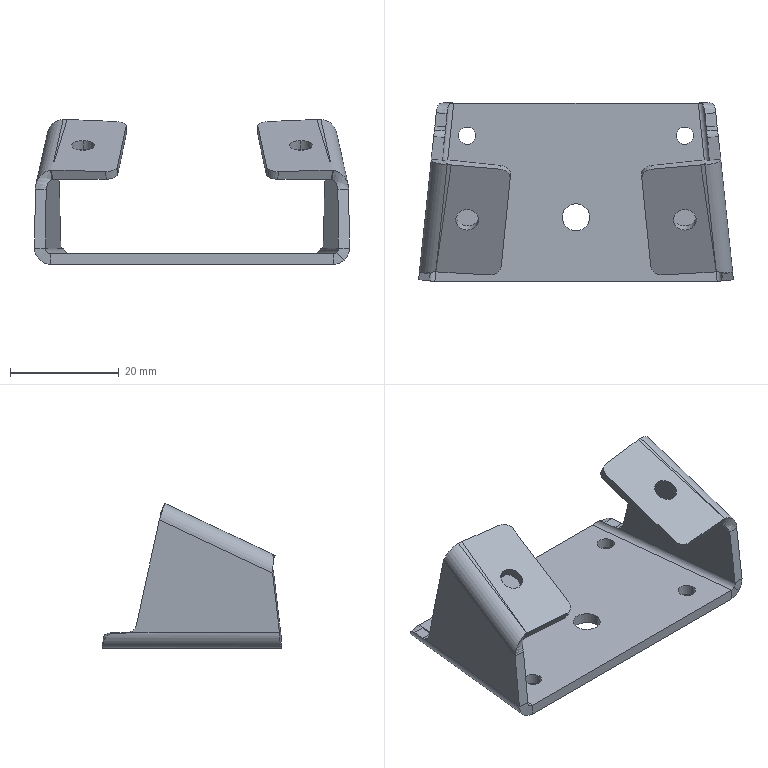Part | SolidWorks | features BaseBody 1 | 1 solid | 73 faces | box 57.881 x 32.818 x 26.649 mm | volume 6139 mm3 | plane 26 | cylinder 24 | spline 23 | commonest cylinder face diameters 3.2 x8 2 x4 4.2 x4 6 x4 4 x2 5 x2